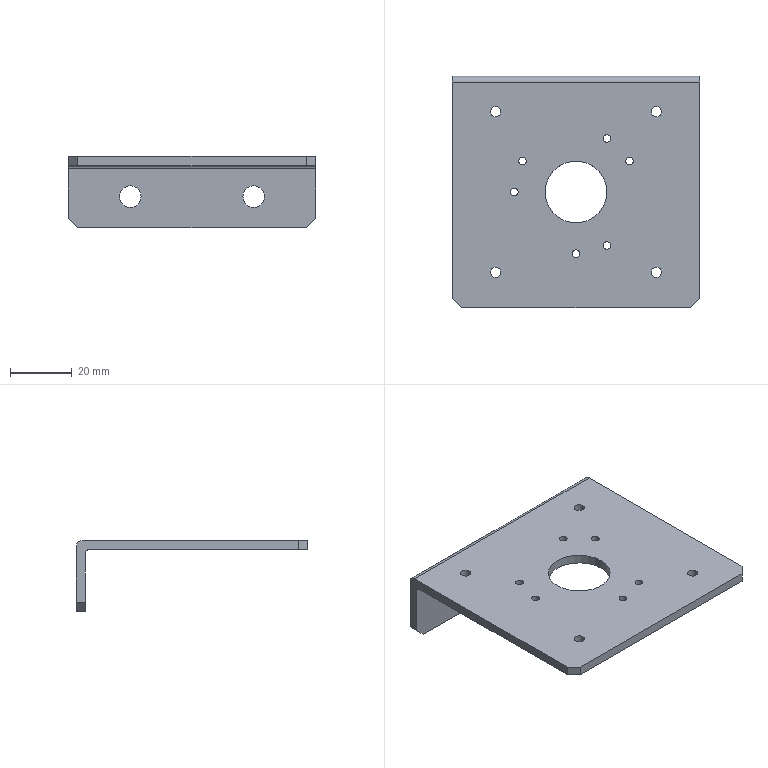Part | NX | 1 solid | 27 faces | box 80 x 75 x 23 mm | volume 21330 mm3 | cylinder 15 | plane 12 | commonest cylinder face diameters 2.5 x6 3.3 x4 7 x2 2 x1 4 x1 20 x1
STEP:
#1=CARTESIAN_POINT('',(10.,0.,-1.5));
#2=VERTEX_POINT('',#1);
#3=CARTESIAN_POINT('',(0.,0.,-1.5));
#4=DIRECTION('',(0.,0.,1.));
#5=DIRECTION('',(1.,0.,0.));
#6=AXIS2_PLACEMENT_3D('',#3,#4,#5);
#7=CIRCLE('',#6,10.);
#8=EDGE_CURVE('',#2,#2,#7,.T.);
#9=ORIENTED_EDGE('',*,*,#8,.T.);
#10=EDGE_LOOP('',(#9));
#11=FACE_BOUND('',#10,.T.);
#12=CARTESIAN_POINT('',(-24.35,-26.,-1.5));
#13=VERTEX_POINT('',#12);
#14=CARTESIAN_POINT('',(-26.,-26.,-1.5));
#15=DIRECTION('',(0.,0.,1.));
#16=DIRECTION('',(1.,0.,0.));
#17=AXIS2_PLACEMENT_3D('',#14,#15,#16);
#18=CIRCLE('',#17,1.65);
#19=EDGE_CURVE('',#13,#13,#18,.T.);
#20=ORIENTED_EDGE('',*,*,#19,.T.);
#21=EDGE_LOOP('',(#20));
#22=FACE_BOUND('',#21,.T.);
#23=CARTESIAN_POINT('',(27.65,-26.,-1.5));
#24=VERTEX_POINT('',#23);
#25=CARTESIAN_POINT('',(26.,-26.,-1.5));
#26=DIRECTION('',(0.,0.,1.));
#27=DIRECTION('',(1.,0.,0.));
#28=AXIS2_PLACEMENT_3D('',#25,#26,#27);
#29=CIRCLE('',#28,1.65);
#30=EDGE_CURVE('',#24,#24,#29,.T.);
#31=ORIENTED_EDGE('',*,*,#30,.T.);
#32=EDGE_LOOP('',(#31));
#33=FACE_BOUND('',#32,.T.);
#34=CARTESIAN_POINT('',(27.65,26.,-1.5));
#35=VERTEX_POINT('',#34);
#36=CARTESIAN_POINT('',(26.,26.,-1.5));
#37=DIRECTION('',(0.,0.,1.));
#38=DIRECTION('',(1.,0.,0.));
#39=AXIS2_PLACEMENT_3D('',#36,#37,#38);
#40=CIRCLE('',#39,1.65);
#41=EDGE_CURVE('',#35,#35,#40,.T.);
#42=ORIENTED_EDGE('',*,*,#41,.T.);
#43=EDGE_LOOP('',(#42));
#44=FACE_BOUND('',#43,.T.);
#45=CARTESIAN_POINT('',(-24.35,26.,-1.5));
#46=VERTEX_POINT('',#45);
#47=CARTESIAN_POINT('',(-26.,26.,-1.5));
#48=DIRECTION('',(0.,0.,1.));
#49=DIRECTION('',(1.,0.,0.));
#50=AXIS2_PLACEMENT_3D('',#47,#48,#49);
#51=CIRCLE('',#50,1.65);
#52=EDGE_CURVE('',#46,#46,#51,.T.);
#53=ORIENTED_EDGE('',*,*,#52,.T.);
#54=EDGE_LOOP('',(#53));
#55=FACE_BOUND('',#54,.T.);
#56=CARTESIAN_POINT('',(1.25,-20.,-1.5));
#57=VERTEX_POINT('',#56);
#58=CARTESIAN_POINT('',(0.,-20.,-1.5));
#59=DIRECTION('',(0.,0.,1.));
#60=DIRECTION('',(1.,0.,0.));
#61=AXIS2_PLACEMENT_3D('',#58,#59,#60);
#62=CIRCLE('',#61,1.25);
#63=EDGE_CURVE('',#57,#57,#62,.T.);
#64=ORIENTED_EDGE('',*,*,#63,.T.);
#65=EDGE_LOOP('',(#64));
#66=FACE_BOUND('',#65,.T.);
#67=CARTESIAN_POINT('',(18.571,10.,-1.5));
#68=VERTEX_POINT('',#67);
#69=CARTESIAN_POINT('',(17.321,10.,-1.5));
#70=DIRECTION('',(0.,0.,1.));
#71=DIRECTION('',(1.,0.,0.));
#72=AXIS2_PLACEMENT_3D('',#69,#70,#71);
#73=CIRCLE('',#72,1.25);
#74=EDGE_CURVE('',#68,#68,#73,.T.);
#75=ORIENTED_EDGE('',*,*,#74,.T.);
#76=EDGE_LOOP('',(#75));
#77=FACE_BOUND('',#76,.T.);
#78=CARTESIAN_POINT('',(-16.071,10.,-1.5));
#79=VERTEX_POINT('',#78);
#80=CARTESIAN_POINT('',(-17.321,10.,-1.5));
#81=DIRECTION('',(0.,0.,1.));
#82=DIRECTION('',(1.,0.,0.));
#83=AXIS2_PLACEMENT_3D('',#80,#81,#82);
#84=CIRCLE('',#83,1.25);
#85=EDGE_CURVE('',#79,#79,#84,.T.);
#86=ORIENTED_EDGE('',*,*,#85,.T.);
#87=EDGE_LOOP('',(#86));
#88=FACE_BOUND('',#87,.T.);
#89=CARTESIAN_POINT('',(10.,16.071,-1.5));
#90=VERTEX_POINT('',#89);
#91=CARTESIAN_POINT('',(10.,17.321,-1.5));
#92=DIRECTION('',(0.,0.,1.));
#93=DIRECTION('',(0.,-1.,0.));
#94=AXIS2_PLACEMENT_3D('',#91,#92,#93);
#95=CIRCLE('',#94,1.25);
#96=EDGE_CURVE('',#90,#90,#95,.T.);
#97=ORIENTED_EDGE('',*,*,#96,.T.);
#98=EDGE_LOOP('',(#97));
#99=FACE_BOUND('',#98,.T.);
#100=CARTESIAN_POINT('',(-20.,-1.25,-1.5));
#101=VERTEX_POINT('',#100);
#102=CARTESIAN_POINT('',(-20.,0.,-1.5));
#103=DIRECTION('',(0.,0.,1.));
#104=DIRECTION('',(0.,-1.,0.));
#105=AXIS2_PLACEMENT_3D('',#102,#103,#104);
#106=CIRCLE('',#105,1.25);
#107=EDGE_CURVE('',#101,#101,#106,.T.);
#108=ORIENTED_EDGE('',*,*,#107,.T.);
#109=EDGE_LOOP('',(#108));
#110=FACE_BOUND('',#109,.T.);
#111=CARTESIAN_POINT('',(10.,-18.571,-1.5));
#112=VERTEX_POINT('',#111);
#113=CARTESIAN_POINT('',(10.,-17.321,-1.5));
#114=DIRECTION('',(0.,0.,1.));
#115=DIRECTION('',(0.,-1.,0.));
#116=AXIS2_PLACEMENT_3D('',#113,#114,#115);
#117=CIRCLE('',#116,1.25);
#118=EDGE_CURVE('',#112,#112,#117,.T.);
#119=ORIENTED_EDGE('',*,*,#118,.T.);
#120=EDGE_LOOP('',(#119));
#121=FACE_BOUND('',#120,.T.);
#122=CARTESIAN_POINT('',(-37.,-37.5,-1.5));
#123=VERTEX_POINT('',#122);
#124=CARTESIAN_POINT('',(37.,-37.5,-1.5));
#125=VERTEX_POINT('',#124);
#126=CARTESIAN_POINT('',(-40.,-37.5,-1.5));
#127=DIRECTION('',(1.,0.,0.));
#128=VECTOR('',#127,1000.);
#129=LINE('',#126,#128);
#130=EDGE_CURVE('',#123,#125,#129,.T.);
#131=ORIENTED_EDGE('',*,*,#130,.F.);
#132=CARTESIAN_POINT('',(-40.,-34.5,-1.5));
#133=VERTEX_POINT('',#132);
#134=CARTESIAN_POINT('',(-37.,-37.5,-1.5));
#135=DIRECTION('',(0.7071,-0.7071,0.));
#136=VECTOR('',#135,1000.);
#137=LINE('',#134,#136);
#138=EDGE_CURVE('',#123,#133,#137,.F.);
#139=ORIENTED_EDGE('',*,*,#138,.T.);
#140=CARTESIAN_POINT('',(-40.,33.5,-1.5));
#141=VERTEX_POINT('',#140);
#142=CARTESIAN_POINT('',(-40.,37.5,-1.5));
#143=DIRECTION('',(0.,-1.,0.));
#144=VECTOR('',#143,1000.);
#145=LINE('',#142,#144);
#146=EDGE_CURVE('',#141,#133,#145,.T.);
#147=ORIENTED_EDGE('',*,*,#146,.F.);
#148=CARTESIAN_POINT('',(40.,33.5,-1.5));
#149=VERTEX_POINT('',#148);
#150=CARTESIAN_POINT('',(40.,33.5,-1.5));
#151=DIRECTION('',(-1.,0.,0.));
#152=VECTOR('',#151,1000.);
#153=LINE('',#150,#152);
#154=EDGE_CURVE('',#141,#149,#153,.F.);
#155=ORIENTED_EDGE('',*,*,#154,.T.);
#156=CARTESIAN_POINT('',(40.,-34.5,-1.5));
#157=VERTEX_POINT('',#156);
#158=CARTESIAN_POINT('',(40.,37.5,-1.5));
#159=DIRECTION('',(0.,1.,0.));
#160=VECTOR('',#159,1000.);
#161=LINE('',#158,#160);
#162=EDGE_CURVE('',#157,#149,#161,.T.);
#163=ORIENTED_EDGE('',*,*,#162,.F.);
#164=CARTESIAN_POINT('',(40.,-34.5,-1.5));
#165=DIRECTION('',(0.7071,0.7071,0.));
#166=VECTOR('',#165,1000.);
#167=LINE('',#164,#166);
#168=EDGE_CURVE('',#157,#125,#167,.F.);
#169=ORIENTED_EDGE('',*,*,#168,.T.);
#170=EDGE_LOOP('',(#131,#139,#147,#155,#163,#169));
#171=FACE_BOUND('',#170,.T.);
#172=CARTESIAN_POINT('',(0.,0.,-1.5));
#173=DIRECTION('',(0.,0.,1.));
#174=DIRECTION('',(1.,0.,0.));
#175=AXIS2_PLACEMENT_3D('',#172,#173,#174);
#176=PLANE('',#175);
#177=ADVANCED_FACE('',(#11,#22,#33,#44,#55,#66,#77,#88,#99,#110,#121,#171),#176,.F.);
#178=CARTESIAN_POINT('',(10.,-18.571,1.5));
#179=VERTEX_POINT('',#178);
#180=CARTESIAN_POINT('',(10.,-17.321,1.5));
#181=DIRECTION('',(0.,0.,1.));
#182=DIRECTION('',(0.,-1.,0.));
#183=AXIS2_PLACEMENT_3D('',#180,#181,#182);
#184=CIRCLE('',#183,1.25);
#185=EDGE_CURVE('',#179,#179,#184,.T.);
#186=ORIENTED_EDGE('',*,*,#185,.F.);
#187=EDGE_LOOP('',(#186));
#188=FACE_BOUND('',#187,.T.);
#189=CARTESIAN_POINT('',(-20.,-1.25,1.5));
#190=VERTEX_POINT('',#189);
#191=CARTESIAN_POINT('',(-20.,0.,1.5));
#192=DIRECTION('',(0.,0.,1.));
#193=DIRECTION('',(0.,-1.,0.));
#194=AXIS2_PLACEMENT_3D('',#191,#192,#193);
#195=CIRCLE('',#194,1.25);
#196=EDGE_CURVE('',#190,#190,#195,.T.);
#197=ORIENTED_EDGE('',*,*,#196,.F.);
#198=EDGE_LOOP('',(#197));
#199=FACE_BOUND('',#198,.T.);
#200=CARTESIAN_POINT('',(10.,16.071,1.5));
#201=VERTEX_POINT('',#200);
#202=CARTESIAN_POINT('',(10.,17.321,1.5));
#203=DIRECTION('',(0.,0.,1.));
#204=DIRECTION('',(0.,-1.,0.));
#205=AXIS2_PLACEMENT_3D('',#202,#203,#204);
#206=CIRCLE('',#205,1.25);
#207=EDGE_CURVE('',#201,#201,#206,.T.);
#208=ORIENTED_EDGE('',*,*,#207,.F.);
#209=EDGE_LOOP('',(#208));
#210=FACE_BOUND('',#209,.T.);
#211=CARTESIAN_POINT('',(-16.071,10.,1.5));
#212=VERTEX_POINT('',#211);
#213=CARTESIAN_POINT('',(-17.321,10.,1.5));
#214=DIRECTION('',(0.,0.,1.));
#215=DIRECTION('',(1.,0.,0.));
#216=AXIS2_PLACEMENT_3D('',#213,#214,#215);
#217=CIRCLE('',#216,1.25);
#218=EDGE_CURVE('',#212,#212,#217,.T.);
#219=ORIENTED_EDGE('',*,*,#218,.F.);
#220=EDGE_LOOP('',(#219));
#221=FACE_BOUND('',#220,.T.);
#222=CARTESIAN_POINT('',(18.571,10.,1.5));
#223=VERTEX_POINT('',#222);
#224=CARTESIAN_POINT('',(17.321,10.,1.5));
#225=DIRECTION('',(0.,0.,1.));
#226=DIRECTION('',(1.,0.,0.));
#227=AXIS2_PLACEMENT_3D('',#224,#225,#226);
#228=CIRCLE('',#227,1.25);
#229=EDGE_CURVE('',#223,#223,#228,.T.);
#230=ORIENTED_EDGE('',*,*,#229,.F.);
#231=EDGE_LOOP('',(#230));
#232=FACE_BOUND('',#231,.T.);
#233=CARTESIAN_POINT('',(1.25,-20.,1.5));
#234=VERTEX_POINT('',#233);
#235=CARTESIAN_POINT('',(0.,-20.,1.5));
#236=DIRECTION('',(0.,0.,1.));
#237=DIRECTION('',(1.,0.,0.));
#238=AXIS2_PLACEMENT_3D('',#235,#236,#237);
#239=CIRCLE('',#238,1.25);
#240=EDGE_CURVE('',#234,#234,#239,.T.);
#241=ORIENTED_EDGE('',*,*,#240,.F.);
#242=EDGE_LOOP('',(#241));
#243=FACE_BOUND('',#242,.T.);
#244=CARTESIAN_POINT('',(-24.35,26.,1.5));
#245=VERTEX_POINT('',#244);
#246=CARTESIAN_POINT('',(-26.,26.,1.5));
#247=DIRECTION('',(0.,0.,1.));
#248=DIRECTION('',(1.,0.,0.));
#249=AXIS2_PLACEMENT_3D('',#246,#247,#248);
#250=CIRCLE('',#249,1.65);
#251=EDGE_CURVE('',#245,#245,#250,.T.);
#252=ORIENTED_EDGE('',*,*,#251,.F.);
#253=EDGE_LOOP('',(#252));
#254=FACE_BOUND('',#253,.T.);
#255=CARTESIAN_POINT('',(27.65,26.,1.5));
#256=VERTEX_POINT('',#255);
#257=CARTESIAN_POINT('',(26.,26.,1.5));
#258=DIRECTION('',(0.,0.,1.));
#259=DIRECTION('',(1.,0.,0.));
#260=AXIS2_PLACEMENT_3D('',#257,#258,#259);
#261=CIRCLE('',#260,1.65);
#262=EDGE_CURVE('',#256,#256,#261,.T.);
#263=ORIENTED_EDGE('',*,*,#262,.F.);
#264=EDGE_LOOP('',(#263));
#265=FACE_BOUND('',#264,.T.);
#266=CARTESIAN_POINT('',(27.65,-26.,1.5));
#267=VERTEX_POINT('',#266);
#268=CARTESIAN_POINT('',(26.,-26.,1.5));
#269=DIRECTION('',(0.,0.,1.));
#270=DIRECTION('',(1.,0.,0.));
#271=AXIS2_PLACEMENT_3D('',#268,#269,#270);
#272=CIRCLE('',#271,1.65);
#273=EDGE_CURVE('',#267,#267,#272,.T.);
#274=ORIENTED_EDGE('',*,*,#273,.F.);
#275=EDGE_LOOP('',(#274));
#276=FACE_BOUND('',#275,.T.);
#277=CARTESIAN_POINT('',(-24.35,-26.,1.5));
#278=VERTEX_POINT('',#277);
#279=CARTESIAN_POINT('',(-26.,-26.,1.5));
#280=DIRECTION('',(0.,0.,1.));
#281=DIRECTION('',(1.,0.,0.));
#282=AXIS2_PLACEMENT_3D('',#279,#280,#281);
#283=CIRCLE('',#282,1.65);
#284=EDGE_CURVE('',#278,#278,#283,.T.);
#285=ORIENTED_EDGE('',*,*,#284,.F.);
#286=EDGE_LOOP('',(#285));
#287=FACE_BOUND('',#286,.T.);
#288=CARTESIAN_POINT('',(-40.,35.5,1.5));
#289=VERTEX_POINT('',#288);
#290=CARTESIAN_POINT('',(-40.,-34.5,1.5));
#291=VERTEX_POINT('',#290);
#292=CARTESIAN_POINT('',(-40.,37.5,1.5));
#293=DIRECTION('',(0.,-1.,0.));
#294=VECTOR('',#293,1000.);
#295=LINE('',#292,#294);
#296=EDGE_CURVE('',#289,#291,#295,.T.);
#297=ORIENTED_EDGE('',*,*,#296,.T.);
#298=CARTESIAN_POINT('',(-37.,-37.5,1.5));
#299=VERTEX_POINT('',#298);
#300=CARTESIAN_POINT('',(-37.25,-37.25,1.5));
#301=DIRECTION('',(-0.7071,0.7071,0.));
#302=VECTOR('',#301,1000.);
#303=LINE('',#300,#302);
#304=EDGE_CURVE('',#291,#299,#303,.F.);
#305=ORIENTED_EDGE('',*,*,#304,.T.);
#306=CARTESIAN_POINT('',(37.,-37.5,1.5));
#307=VERTEX_POINT('',#306);
#308=CARTESIAN_POINT('',(-40.,-37.5,1.5));
#309=DIRECTION('',(1.,0.,0.));
#310=VECTOR('',#309,1000.);
#311=LINE('',#308,#310);
#312=EDGE_CURVE('',#299,#307,#311,.T.);
#313=ORIENTED_EDGE('',*,*,#312,.T.);
#314=CARTESIAN_POINT('',(40.,-34.5,1.5));
#315=VERTEX_POINT('',#314);
#316=CARTESIAN_POINT('',(37.25,-37.25,1.5));
#317=DIRECTION('',(-0.7071,-0.7071,0.));
#318=VECTOR('',#317,1000.);
#319=LINE('',#316,#318);
#320=EDGE_CURVE('',#307,#315,#319,.F.);
#321=ORIENTED_EDGE('',*,*,#320,.T.);
#322=CARTESIAN_POINT('',(40.,35.5,1.5));
#323=VERTEX_POINT('',#322);
#324=CARTESIAN_POINT('',(40.,37.5,1.5));
#325=DIRECTION('',(0.,1.,0.));
#326=VECTOR('',#325,1000.);
#327=LINE('',#324,#326);
#328=EDGE_CURVE('',#315,#323,#327,.T.);
#329=ORIENTED_EDGE('',*,*,#328,.T.);
#330=CARTESIAN_POINT('',(-40.,35.5,1.5));
#331=DIRECTION('',(-1.,0.,0.));
#332=VECTOR('',#331,1000.);
#333=LINE('',#330,#332);
#334=EDGE_CURVE('',#323,#289,#333,.T.);
#335=ORIENTED_EDGE('',*,*,#334,.T.);
#336=EDGE_LOOP('',(#297,#305,#313,#321,#329,#335));
#337=FACE_BOUND('',#336,.T.);
#338=CARTESIAN_POINT('',(10.,0.,1.5));
#339=VERTEX_POINT('',#338);
#340=CARTESIAN_POINT('',(0.,0.,1.5));
#341=DIRECTION('',(0.,0.,1.));
#342=DIRECTION('',(1.,0.,0.));
#343=AXIS2_PLACEMENT_3D('',#340,#341,#342);
#344=CIRCLE('',#343,10.);
#345=EDGE_CURVE('',#339,#339,#344,.T.);
#346=ORIENTED_EDGE('',*,*,#345,.F.);
#347=EDGE_LOOP('',(#346));
#348=FACE_BOUND('',#347,.T.);
#349=CARTESIAN_POINT('',(0.,0.,1.5));
#350=DIRECTION('',(0.,0.,1.));
#351=DIRECTION('',(1.,0.,0.));
#352=AXIS2_PLACEMENT_3D('',#349,#350,#351);
#353=PLANE('',#352);
#354=ADVANCED_FACE('',(#188,#199,#210,#221,#232,#243,#254,#265,#276,#287,#337,#348),#353,.T.);
#355=ORIENTED_EDGE('',*,*,#328,.F.);
#356=CARTESIAN_POINT('',(40.,-34.5,1.5));
#357=DIRECTION('',(0.,0.,-1.));
#358=VECTOR('',#357,1000.);
#359=LINE('',#356,#358);
#360=EDGE_CURVE('',#315,#157,#359,.T.);
#361=ORIENTED_EDGE('',*,*,#360,.T.);
#362=ORIENTED_EDGE('',*,*,#162,.T.);
#363=CARTESIAN_POINT('',(40.,34.5,-2.5));
#364=VERTEX_POINT('',#363);
#365=CARTESIAN_POINT('',(40.,33.5,-2.5));
#366=DIRECTION('',(-1.,0.,0.));
#367=DIRECTION('',(0.,-1.,0.));
#368=AXIS2_PLACEMENT_3D('',#365,#366,#367);
#369=CIRCLE('',#368,1.);
#370=EDGE_CURVE('',#149,#364,#369,.T.);
#371=ORIENTED_EDGE('',*,*,#370,.T.);
#372=CARTESIAN_POINT('',(40.,34.5,-18.5));
#373=VERTEX_POINT('',#372);
#374=CARTESIAN_POINT('',(40.,34.5,-21.5));
#375=DIRECTION('',(0.,0.,1.));
#376=VECTOR('',#375,1000.);
#377=LINE('',#374,#376);
#378=EDGE_CURVE('',#373,#364,#377,.T.);
#379=ORIENTED_EDGE('',*,*,#378,.F.);
#380=CARTESIAN_POINT('',(40.,37.5,-18.5));
#381=VERTEX_POINT('',#380);
#382=CARTESIAN_POINT('',(40.,37.5,-18.5));
#383=DIRECTION('',(0.,1.,0.));
#384=VECTOR('',#383,1000.);
#385=LINE('',#382,#384);
#386=EDGE_CURVE('',#373,#381,#385,.T.);
#387=ORIENTED_EDGE('',*,*,#386,.T.);
#388=CARTESIAN_POINT('',(40.,37.5,-0.5));
#389=VERTEX_POINT('',#388);
#390=CARTESIAN_POINT('',(40.,37.5,1.5));
#391=DIRECTION('',(0.,0.,-1.));
#392=VECTOR('',#391,1000.);
#393=LINE('',#390,#392);
#394=EDGE_CURVE('',#389,#381,#393,.T.);
#395=ORIENTED_EDGE('',*,*,#394,.F.);
#396=CARTESIAN_POINT('',(40.,35.5,-0.5));
#397=DIRECTION('',(-1.,0.,0.));
#398=DIRECTION('',(0.,-1.,0.));
#399=AXIS2_PLACEMENT_3D('',#396,#397,#398);
#400=CIRCLE('',#399,2.);
#401=EDGE_CURVE('',#389,#323,#400,.F.);
#402=ORIENTED_EDGE('',*,*,#401,.T.);
#403=EDGE_LOOP('',(#355,#361,#362,#371,#379,#387,#395,#402));
#404=FACE_BOUND('',#403,.T.);
#405=CARTESIAN_POINT('',(40.,37.5,1.5));
#406=DIRECTION('',(-1.,0.,0.));
#407=DIRECTION('',(0.,-1.,0.));
#408=AXIS2_PLACEMENT_3D('',#405,#406,#407);
#409=PLANE('',#408);
#410=ADVANCED_FACE('',(#404),#409,.F.);
#411=CARTESIAN_POINT('',(23.5,37.5,-11.5));
#412=VERTEX_POINT('',#411);
#413=CARTESIAN_POINT('',(20.,37.5,-11.5));
#414=DIRECTION('',(0.,-1.,0.));
#415=DIRECTION('',(1.,0.,0.));
#416=AXIS2_PLACEMENT_3D('',#413,#414,#415);
#417=CIRCLE('',#416,3.5);
#418=EDGE_CURVE('',#412,#412,#417,.T.);
#419=ORIENTED_EDGE('',*,*,#418,.T.);
#420=EDGE_LOOP('',(#419));
#421=FACE_BOUND('',#420,.T.);
#422=CARTESIAN_POINT('',(-16.5,37.5,-11.5));
#423=VERTEX_POINT('',#422);
#424=CARTESIAN_POINT('',(-20.,37.5,-11.5));
#425=DIRECTION('',(0.,-1.,0.));
#426=DIRECTION('',(1.,0.,0.));
#427=AXIS2_PLACEMENT_3D('',#424,#425,#426);
#428=CIRCLE('',#427,3.5);
#429=EDGE_CURVE('',#423,#423,#428,.T.);
#430=ORIENTED_EDGE('',*,*,#429,.T.);
#431=EDGE_LOOP('',(#430));
#432=FACE_BOUND('',#431,.T.);
#433=ORIENTED_EDGE('',*,*,#394,.T.);
#434=CARTESIAN_POINT('',(37.,37.5,-21.5));
#435=VERTEX_POINT('',#434);
#436=CARTESIAN_POINT('',(37.,37.5,-21.5));
#437=DIRECTION('',(0.7071,0.,0.7071));
#438=VECTOR('',#437,1000.);
#439=LINE('',#436,#438);
#440=EDGE_CURVE('',#381,#435,#439,.F.);
#441=ORIENTED_EDGE('',*,*,#440,.T.);
#442=CARTESIAN_POINT('',(-37.,37.5,-21.5));
#443=VERTEX_POINT('',#442);
#444=CARTESIAN_POINT('',(-40.,37.5,-21.5));
#445=DIRECTION('',(1.,0.,0.));
#446=VECTOR('',#445,1000.);
#447=LINE('',#444,#446);
#448=EDGE_CURVE('',#443,#435,#447,.T.);
#449=ORIENTED_EDGE('',*,*,#448,.F.);
#450=CARTESIAN_POINT('',(-40.,37.5,-18.5));
#451=VERTEX_POINT('',#450);
#452=CARTESIAN_POINT('',(-37.,37.5,-21.5));
#453=DIRECTION('',(0.7071,0.,-0.7071));
#454=VECTOR('',#453,1000.);
#455=LINE('',#452,#454);
#456=EDGE_CURVE('',#443,#451,#455,.F.);
#457=ORIENTED_EDGE('',*,*,#456,.T.);
#458=CARTESIAN_POINT('',(-40.,37.5,-0.5));
#459=VERTEX_POINT('',#458);
#460=CARTESIAN_POINT('',(-40.,37.5,1.5));
#461=DIRECTION('',(0.,0.,-1.));
#462=VECTOR('',#461,1000.);
#463=LINE('',#460,#462);
#464=EDGE_CURVE('',#459,#451,#463,.T.);
#465=ORIENTED_EDGE('',*,*,#464,.F.);
#466=CARTESIAN_POINT('',(40.,37.5,-0.5));
#467=DIRECTION('',(-1.,0.,0.));
#468=VECTOR('',#467,1000.);
#469=LINE('',#466,#468);
#470=EDGE_CURVE('',#459,#389,#469,.F.);
#471=ORIENTED_EDGE('',*,*,#470,.T.);
#472=EDGE_LOOP('',(#433,#441,#449,#457,#465,#471));
#473=FACE_BOUND('',#472,.T.);
#474=CARTESIAN_POINT('',(-40.,37.5,1.5));
#475=DIRECTION('',(0.,-1.,0.));
#476=DIRECTION('',(0.,0.,-1.));
#477=AXIS2_PLACEMENT_3D('',#474,#475,#476);
#478=PLANE('',#477);
#479=ADVANCED_FACE('',(#421,#432,#473),#478,.F.);
#480=ORIENTED_EDGE('',*,*,#146,.T.);
#481=CARTESIAN_POINT('',(-40.,-34.5,1.5));
#482=DIRECTION('',(0.,0.,1.));
#483=VECTOR('',#482,1000.);
#484=LINE('',#481,#483);
#485=EDGE_CURVE('',#133,#291,#484,.T.);
#486=ORIENTED_EDGE('',*,*,#485,.T.);
#487=ORIENTED_EDGE('',*,*,#296,.F.);
#488=CARTESIAN_POINT('',(-40.,35.5,-0.5));
#489=DIRECTION('',(1.,0.,0.));
#490=DIRECTION('',(0.,1.,0.));
#491=AXIS2_PLACEMENT_3D('',#488,#489,#490);
#492=CIRCLE('',#491,2.);
#493=EDGE_CURVE('',#289,#459,#492,.F.);
#494=ORIENTED_EDGE('',*,*,#493,.T.);
#495=ORIENTED_EDGE('',*,*,#464,.T.);
#496=CARTESIAN_POINT('',(-40.,34.5,-18.5));
#497=VERTEX_POINT('',#496);
#498=CARTESIAN_POINT('',(-40.,37.5,-18.5));
#499=DIRECTION('',(0.,-1.,0.));
#500=VECTOR('',#499,1000.);
#501=LINE('',#498,#500);
#502=EDGE_CURVE('',#451,#497,#501,.T.);
#503=ORIENTED_EDGE('',*,*,#502,.T.);
#504=CARTESIAN_POINT('',(-40.,34.5,-2.5));
#505=VERTEX_POINT('',#504);
#506=CARTESIAN_POINT('',(-40.,34.5,-21.5));
#507=DIRECTION('',(0.,0.,1.));
#508=VECTOR('',#507,1000.);
#509=LINE('',#506,#508);
#510=EDGE_CURVE('',#497,#505,#509,.T.);
#511=ORIENTED_EDGE('',*,*,#510,.T.);
#512=CARTESIAN_POINT('',(-40.,33.5,-2.5));
#513=DIRECTION('',(1.,0.,0.));
#514=DIRECTION('',(0.,1.,0.));
#515=AXIS2_PLACEMENT_3D('',#512,#513,#514);
#516=CIRCLE('',#515,1.);
#517=EDGE_CURVE('',#505,#141,#516,.T.);
#518=ORIENTED_EDGE('',*,*,#517,.T.);
#519=EDGE_LOOP('',(#480,#486,#487,#494,#495,#503,#511,#518));
#520=FACE_BOUND('',#519,.T.);
#521=CARTESIAN_POINT('',(-40.,37.5,1.5));
#522=DIRECTION('',(1.,0.,0.));
#523=DIRECTION('',(0.,1.,0.));
#524=AXIS2_PLACEMENT_3D('',#521,#522,#523);
#525=PLANE('',#524);
#526=ADVANCED_FACE('',(#520),#525,.F.);
#527=ORIENTED_EDGE('',*,*,#312,.F.);
#528=CARTESIAN_POINT('',(-37.,-37.5,1.5));
#529=DIRECTION('',(0.,0.,-1.));
#530=VECTOR('',#529,1000.);
#531=LINE('',#528,#530);
#532=EDGE_CURVE('',#299,#123,#531,.T.);
#533=ORIENTED_EDGE('',*,*,#532,.T.);
#534=ORIENTED_EDGE('',*,*,#130,.T.);
#535=CARTESIAN_POINT('',(37.,-37.5,1.5));
#536=DIRECTION('',(0.,0.,1.));
#537=VECTOR('',#536,1000.);
#538=LINE('',#535,#537);
#539=EDGE_CURVE('',#125,#307,#538,.T.);
#540=ORIENTED_EDGE('',*,*,#539,.T.);
#541=EDGE_LOOP('',(#527,#533,#534,#540));
#542=FACE_BOUND('',#541,.T.);
#543=CARTESIAN_POINT('',(-40.,-37.5,1.5));
#544=DIRECTION('',(0.,1.,0.));
#545=DIRECTION('',(0.,0.,1.));
#546=AXIS2_PLACEMENT_3D('',#543,#544,#545);
#547=PLANE('',#546);
#548=ADVANCED_FACE('',(#542),#547,.F.);
#549=ORIENTED_EDGE('',*,*,#345,.T.);
#550=EDGE_LOOP('',(#549));
#551=FACE_BOUND('',#550,.T.);
#552=ORIENTED_EDGE('',*,*,#8,.F.);
#553=EDGE_LOOP('',(#552));
#554=FACE_BOUND('',#553,.T.);
#555=CARTESIAN_POINT('',(0.,0.,1.5));
#556=DIRECTION('',(0.,0.,-1.));
#557=DIRECTION('',(-1.,0.,0.));
#558=AXIS2_PLACEMENT_3D('',#555,#556,#557);
#559=CYLINDRICAL_SURFACE('',#558,10.);
#560=ADVANCED_FACE('',(#551,#554),#559,.F.);
#561=ORIENTED_EDGE('',*,*,#19,.F.);
#562=EDGE_LOOP('',(#561));
#563=FACE_BOUND('',#562,.T.);
#564=ORIENTED_EDGE('',*,*,#284,.T.);
#565=EDGE_LOOP('',(#564));
#566=FACE_BOUND('',#565,.T.);
#567=CARTESIAN_POINT('',(-26.,-26.,1.5));
#568=DIRECTION('',(0.,0.,1.));
#569=DIRECTION('',(1.,0.,0.));
#570=AXIS2_PLACEMENT_3D('',#567,#568,#569);
#571=CYLINDRICAL_SURFACE('',#570,1.65);
#572=ADVANCED_FACE('',(#563,#566),#571,.F.);
#573=ORIENTED_EDGE('',*,*,#30,.F.);
#574=EDGE_LOOP('',(#573));
#575=FACE_BOUND('',#574,.T.);
#576=ORIENTED_EDGE('',*,*,#273,.T.);
#577=EDGE_LOOP('',(#576));
#578=FACE_BOUND('',#577,.T.);
#579=CARTESIAN_POINT('',(26.,-26.,1.5));
#580=DIRECTION('',(0.,0.,1.));
#581=DIRECTION('',(1.,0.,0.));
#582=AXIS2_PLACEMENT_3D('',#579,#580,#581);
#583=CYLINDRICAL_SURFACE('',#582,1.65);
#584=ADVANCED_FACE('',(#575,#578),#583,.F.);
#585=ORIENTED_EDGE('',*,*,#41,.F.);
#586=EDGE_LOOP('',(#585));
#587=FACE_BOUND('',#586,.T.);
#588=ORIENTED_EDGE('',*,*,#262,.T.);
#589=EDGE_LOOP('',(#588));
#590=FACE_BOUND('',#589,.T.);
#591=CARTESIAN_POINT('',(26.,26.,1.5));
#592=DIRECTION('',(0.,0.,1.));
#593=DIRECTION('',(1.,0.,0.));
#594=AXIS2_PLACEMENT_3D('',#591,#592,#593);
#595=CYLINDRICAL_SURFACE('',#594,1.65);
#596=ADVANCED_FACE('',(#587,#590),#595,.F.);
#597=ORIENTED_EDGE('',*,*,#52,.F.);
#598=EDGE_LOOP('',(#597));
#599=FACE_BOUND('',#598,.T.);
#600=ORIENTED_EDGE('',*,*,#251,.T.);
#601=EDGE_LOOP('',(#600));
#602=FACE_BOUND('',#601,.T.);
#603=CARTESIAN_POINT('',(-26.,26.,1.5));
#604=DIRECTION('',(0.,0.,1.));
#605=DIRECTION('',(1.,0.,0.));
#606=AXIS2_PLACEMENT_3D('',#603,#604,#605);
#607=CYLINDRICAL_SURFACE('',#606,1.65);
#608=ADVANCED_FACE('',(#599,#602),#607,.F.);
#609=ORIENTED_EDGE('',*,*,#63,.F.);
#610=EDGE_LOOP('',(#609));
#611=FACE_BOUND('',#610,.T.);
#612=ORIENTED_EDGE('',*,*,#240,.T.);
#613=EDGE_LOOP('',(#612));
#614=FACE_BOUND('',#613,.T.);
#615=CARTESIAN_POINT('',(0.,-20.,1.5));
#616=DIRECTION('',(0.,0.,1.));
#617=DIRECTION('',(1.,0.,0.));
#618=AXIS2_PLACEMENT_3D('',#615,#616,#617);
#619=CYLINDRICAL_SURFACE('',#618,1.25);
#620=ADVANCED_FACE('',(#611,#614),#619,.F.);
#621=ORIENTED_EDGE('',*,*,#74,.F.);
#622=EDGE_LOOP('',(#621));
#623=FACE_BOUND('',#622,.T.);
#624=ORIENTED_EDGE('',*,*,#229,.T.);
#625=EDGE_LOOP('',(#624));
#626=FACE_BOUND('',#625,.T.);
#627=CARTESIAN_POINT('',(17.321,10.,1.5));
#628=DIRECTION('',(0.,0.,1.));
#629=DIRECTION('',(1.,0.,0.));
#630=AXIS2_PLACEMENT_3D('',#627,#628,#629);
#631=CYLINDRICAL_SURFACE('',#630,1.25);
#632=ADVANCED_FACE('',(#623,#626),#631,.F.);
#633=ORIENTED_EDGE('',*,*,#85,.F.);
#634=EDGE_LOOP('',(#633));
#635=FACE_BOUND('',#634,.T.);
#636=ORIENTED_EDGE('',*,*,#218,.T.);
#637=EDGE_LOOP('',(#636));
#638=FACE_BOUND('',#637,.T.);
#639=CARTESIAN_POINT('',(-17.321,10.,1.5));
#640=DIRECTION('',(0.,0.,1.));
#641=DIRECTION('',(1.,0.,0.));
#642=AXIS2_PLACEMENT_3D('',#639,#640,#641);
#643=CYLINDRICAL_SURFACE('',#642,1.25);
#644=ADVANCED_FACE('',(#635,#638),#643,.F.);
#645=ORIENTED_EDGE('',*,*,#96,.F.);
#646=EDGE_LOOP('',(#645));
#647=FACE_BOUND('',#646,.T.);
#648=ORIENTED_EDGE('',*,*,#207,.T.);
#649=EDGE_LOOP('',(#648));
#650=FACE_BOUND('',#649,.T.);
#651=CARTESIAN_POINT('',(10.,17.321,1.5));
#652=DIRECTION('',(0.,0.,1.));
#653=DIRECTION('',(0.,-1.,0.));
#654=AXIS2_PLACEMENT_3D('',#651,#652,#653);
#655=CYLINDRICAL_SURFACE('',#654,1.25);
#656=ADVANCED_FACE('',(#647,#650),#655,.F.);
#657=ORIENTED_EDGE('',*,*,#107,.F.);
#658=EDGE_LOOP('',(#657));
#659=FACE_BOUND('',#658,.T.);
#660=ORIENTED_EDGE('',*,*,#196,.T.);
#661=EDGE_LOOP('',(#660));
#662=FACE_BOUND('',#661,.T.);
#663=CARTESIAN_POINT('',(-20.,0.,1.5));
#664=DIRECTION('',(0.,0.,1.));
#665=DIRECTION('',(0.,-1.,0.));
#666=AXIS2_PLACEMENT_3D('',#663,#664,#665);
#667=CYLINDRICAL_SURFACE('',#666,1.25);
#668=ADVANCED_FACE('',(#659,#662),#667,.F.);
#669=ORIENTED_EDGE('',*,*,#118,.F.);
#670=EDGE_LOOP('',(#669));
#671=FACE_BOUND('',#670,.T.);
#672=ORIENTED_EDGE('',*,*,#185,.T.);
#673=EDGE_LOOP('',(#672));
#674=FACE_BOUND('',#673,.T.);
#675=CARTESIAN_POINT('',(10.,-17.321,1.5));
#676=DIRECTION('',(0.,0.,1.));
#677=DIRECTION('',(0.,-1.,0.));
#678=AXIS2_PLACEMENT_3D('',#675,#676,#677);
#679=CYLINDRICAL_SURFACE('',#678,1.25);
#680=ADVANCED_FACE('',(#671,#674),#679,.F.);
#681=CARTESIAN_POINT('',(23.5,34.5,-11.5));
#682=VERTEX_POINT('',#681);
#683=CARTESIAN_POINT('',(20.,34.5,-11.5));
#684=DIRECTION('',(0.,-1.,0.));
#685=DIRECTION('',(1.,0.,0.));
#686=AXIS2_PLACEMENT_3D('',#683,#684,#685);
#687=CIRCLE('',#686,3.5);
#688=EDGE_CURVE('',#682,#682,#687,.T.);
#689=ORIENTED_EDGE('',*,*,#688,.F.);
#690=EDGE_LOOP('',(#689));
#691=FACE_BOUND('',#690,.T.);
#692=CARTESIAN_POINT('',(-16.5,34.5,-11.5));
#693=VERTEX_POINT('',#692);
#694=CARTESIAN_POINT('',(-20.,34.5,-11.5));
#695=DIRECTION('',(0.,-1.,0.));
#696=DIRECTION('',(1.,0.,0.));
#697=AXIS2_PLACEMENT_3D('',#694,#695,#696);
#698=CIRCLE('',#697,3.5);
#699=EDGE_CURVE('',#693,#693,#698,.T.);
#700=ORIENTED_EDGE('',*,*,#699,.F.);
#701=EDGE_LOOP('',(#700));
#702=FACE_BOUND('',#701,.T.);
#703=CARTESIAN_POINT('',(37.,34.5,-21.5));
#704=VERTEX_POINT('',#703);
#705=CARTESIAN_POINT('',(-37.,34.5,-21.5));
#706=VERTEX_POINT('',#705);
#707=CARTESIAN_POINT('',(-40.,34.5,-21.5));
#708=DIRECTION('',(-1.,0.,0.));
#709=VECTOR('',#708,1000.);
#710=LINE('',#707,#709);
#711=EDGE_CURVE('',#704,#706,#710,.T.);
#712=ORIENTED_EDGE('',*,*,#711,.F.);
#713=CARTESIAN_POINT('',(37.,34.5,-21.5));
#714=DIRECTION('',(-0.7071,0.,-0.7071));
#715=VECTOR('',#714,1000.);
#716=LINE('',#713,#715);
#717=EDGE_CURVE('',#704,#373,#716,.F.);
#718=ORIENTED_EDGE('',*,*,#717,.T.);
#719=ORIENTED_EDGE('',*,*,#378,.T.);
#720=CARTESIAN_POINT('',(-40.,34.5,-2.5));
#721=DIRECTION('',(-1.,0.,0.));
#722=VECTOR('',#721,1000.);
#723=LINE('',#720,#722);
#724=EDGE_CURVE('',#364,#505,#723,.T.);
#725=ORIENTED_EDGE('',*,*,#724,.T.);
#726=ORIENTED_EDGE('',*,*,#510,.F.);
#727=CARTESIAN_POINT('',(-37.,34.5,-21.5));
#728=DIRECTION('',(-0.7071,0.,0.7071));
#729=VECTOR('',#728,1000.);
#730=LINE('',#727,#729);
#731=EDGE_CURVE('',#497,#706,#730,.F.);
#732=ORIENTED_EDGE('',*,*,#731,.T.);
#733=EDGE_LOOP('',(#712,#718,#719,#725,#726,#732));
#734=FACE_BOUND('',#733,.T.);
#735=CARTESIAN_POINT('',(-40.,34.5,-21.5));
#736=DIRECTION('',(0.,1.,0.));
#737=DIRECTION('',(-1.,0.,0.));
#738=AXIS2_PLACEMENT_3D('',#735,#736,#737);
#739=PLANE('',#738);
#740=ADVANCED_FACE('',(#691,#702,#734),#739,.F.);
#741=ORIENTED_EDGE('',*,*,#448,.T.);
#742=CARTESIAN_POINT('',(37.,0.,-21.5));
#743=DIRECTION('',(0.,-1.,0.));
#744=VECTOR('',#743,1000.);
#745=LINE('',#742,#744);
#746=EDGE_CURVE('',#435,#704,#745,.T.);
#747=ORIENTED_EDGE('',*,*,#746,.T.);
#748=ORIENTED_EDGE('',*,*,#711,.T.);
#749=CARTESIAN_POINT('',(-37.,0.,-21.5));
#750=DIRECTION('',(0.,1.,0.));
#751=VECTOR('',#750,1000.);
#752=LINE('',#749,#751);
#753=EDGE_CURVE('',#706,#443,#752,.T.);
#754=ORIENTED_EDGE('',*,*,#753,.T.);
#755=EDGE_LOOP('',(#741,#747,#748,#754));
#756=FACE_BOUND('',#755,.T.);
#757=CARTESIAN_POINT('',(0.,0.,-21.5));
#758=DIRECTION('',(0.,0.,1.));
#759=DIRECTION('',(1.,0.,0.));
#760=AXIS2_PLACEMENT_3D('',#757,#758,#759);
#761=PLANE('',#760);
#762=ADVANCED_FACE('',(#756),#761,.F.);
#763=ORIENTED_EDGE('',*,*,#401,.F.);
#764=ORIENTED_EDGE('',*,*,#470,.F.);
#765=ORIENTED_EDGE('',*,*,#493,.F.);
#766=ORIENTED_EDGE('',*,*,#334,.F.);
#767=EDGE_LOOP('',(#763,#764,#765,#766));
#768=FACE_BOUND('',#767,.T.);
#769=CARTESIAN_POINT('',(0.,35.5,-0.5));
#770=DIRECTION('',(1.,0.,0.));
#771=DIRECTION('',(0.,0.,-1.));
#772=AXIS2_PLACEMENT_3D('',#769,#770,#771);
#773=CYLINDRICAL_SURFACE('',#772,2.);
#774=ADVANCED_FACE('',(#768),#773,.T.);
#775=ORIENTED_EDGE('',*,*,#370,.F.);
#776=ORIENTED_EDGE('',*,*,#154,.F.);
#777=ORIENTED_EDGE('',*,*,#517,.F.);
#778=ORIENTED_EDGE('',*,*,#724,.F.);
#779=EDGE_LOOP('',(#775,#776,#777,#778));
#780=FACE_BOUND('',#779,.T.);
#781=CARTESIAN_POINT('',(-40.,33.5,-2.5));
#782=DIRECTION('',(1.,0.,0.));
#783=DIRECTION('',(0.,1.,0.));
#784=AXIS2_PLACEMENT_3D('',#781,#782,#783);
#785=CYLINDRICAL_SURFACE('',#784,1.);
#786=ADVANCED_FACE('',(#780),#785,.F.);
#787=ORIENTED_EDGE('',*,*,#304,.F.);
#788=ORIENTED_EDGE('',*,*,#485,.F.);
#789=ORIENTED_EDGE('',*,*,#138,.F.);
#790=ORIENTED_EDGE('',*,*,#532,.F.);
#791=EDGE_LOOP('',(#787,#788,#789,#790));
#792=FACE_BOUND('',#791,.T.);
#793=CARTESIAN_POINT('',(-37.,-37.5,1.5));
#794=DIRECTION('',(0.7071,0.7071,0.));
#795=DIRECTION('',(0.,0.,-1.));
#796=AXIS2_PLACEMENT_3D('',#793,#794,#795);
#797=PLANE('',#796);
#798=ADVANCED_FACE('',(#792),#797,.F.);
#799=ORIENTED_EDGE('',*,*,#320,.F.);
#800=ORIENTED_EDGE('',*,*,#539,.F.);
#801=ORIENTED_EDGE('',*,*,#168,.F.);
#802=ORIENTED_EDGE('',*,*,#360,.F.);
#803=EDGE_LOOP('',(#799,#800,#801,#802));
#804=FACE_BOUND('',#803,.T.);
#805=CARTESIAN_POINT('',(40.,-34.5,1.5));
#806=DIRECTION('',(-0.7071,0.7071,0.));
#807=DIRECTION('',(0.,0.,-1.));
#808=AXIS2_PLACEMENT_3D('',#805,#806,#807);
#809=PLANE('',#808);
#810=ADVANCED_FACE('',(#804),#809,.F.);
#811=ORIENTED_EDGE('',*,*,#440,.F.);
#812=ORIENTED_EDGE('',*,*,#386,.F.);
#813=ORIENTED_EDGE('',*,*,#717,.F.);
#814=ORIENTED_EDGE('',*,*,#746,.F.);
#815=EDGE_LOOP('',(#811,#812,#813,#814));
#816=FACE_BOUND('',#815,.T.);
#817=CARTESIAN_POINT('',(37.,0.,-21.5));
#818=DIRECTION('',(-0.7071,0.,0.7071));
#819=DIRECTION('',(0.,-1.,0.));
#820=AXIS2_PLACEMENT_3D('',#817,#818,#819);
#821=PLANE('',#820);
#822=ADVANCED_FACE('',(#816),#821,.F.);
#823=ORIENTED_EDGE('',*,*,#731,.F.);
#824=ORIENTED_EDGE('',*,*,#502,.F.);
#825=ORIENTED_EDGE('',*,*,#456,.F.);
#826=ORIENTED_EDGE('',*,*,#753,.F.);
#827=EDGE_LOOP('',(#823,#824,#825,#826));
#828=FACE_BOUND('',#827,.T.);
#829=CARTESIAN_POINT('',(-37.,0.,-21.5));
#830=DIRECTION('',(0.7071,0.,0.7071));
#831=DIRECTION('',(0.,1.,0.));
#832=AXIS2_PLACEMENT_3D('',#829,#830,#831);
#833=PLANE('',#832);
#834=ADVANCED_FACE('',(#828),#833,.F.);
#835=ORIENTED_EDGE('',*,*,#429,.F.);
#836=EDGE_LOOP('',(#835));
#837=FACE_BOUND('',#836,.T.);
#838=ORIENTED_EDGE('',*,*,#699,.T.);
#839=EDGE_LOOP('',(#838));
#840=FACE_BOUND('',#839,.T.);
#841=CARTESIAN_POINT('',(-20.,37.5,-11.5));
#842=DIRECTION('',(0.,-1.,0.));
#843=DIRECTION('',(1.,0.,0.));
#844=AXIS2_PLACEMENT_3D('',#841,#842,#843);
#845=CYLINDRICAL_SURFACE('',#844,3.5);
#846=ADVANCED_FACE('',(#837,#840),#845,.F.);
#847=ORIENTED_EDGE('',*,*,#418,.F.);
#848=EDGE_LOOP('',(#847));
#849=FACE_BOUND('',#848,.T.);
#850=ORIENTED_EDGE('',*,*,#688,.T.);
#851=EDGE_LOOP('',(#850));
#852=FACE_BOUND('',#851,.T.);
#853=CARTESIAN_POINT('',(20.,37.5,-11.5));
#854=DIRECTION('',(0.,-1.,0.));
#855=DIRECTION('',(1.,0.,0.));
#856=AXIS2_PLACEMENT_3D('',#853,#854,#855);
#857=CYLINDRICAL_SURFACE('',#856,3.5);
#858=ADVANCED_FACE('',(#849,#852),#857,.F.);
#859=CLOSED_SHELL('',(#177,#354,#410,#479,#526,#548,#560,#572,#584,#596,#608,#620,#632,#644,#656,#668,#680,#740,#762,#774,#786,#798,#810,#822,#834,#846,#858));
#860=MANIFOLD_SOLID_BREP('',#859);
#861=(LENGTH_UNIT()NAMED_UNIT(*)SI_UNIT(.MILLI.,.METRE.));
#862=UNCERTAINTY_MEASURE_WITH_UNIT(LENGTH_MEASURE(0.00001),#861,'','');
#863=(NAMED_UNIT(*)PLANE_ANGLE_UNIT()SI_UNIT($,.RADIAN.));
#864=(NAMED_UNIT(*)SI_UNIT($,.STERADIAN.)SOLID_ANGLE_UNIT());
#865=(GEOMETRIC_REPRESENTATION_CONTEXT(3)GLOBAL_UNCERTAINTY_ASSIGNED_CONTEXT((#862))GLOBAL_UNIT_ASSIGNED_CONTEXT((#861,#863,#864))REPRESENTATION_CONTEXT('',''));
#866=ADVANCED_BREP_SHAPE_REPRESENTATION('',(#860),#865);